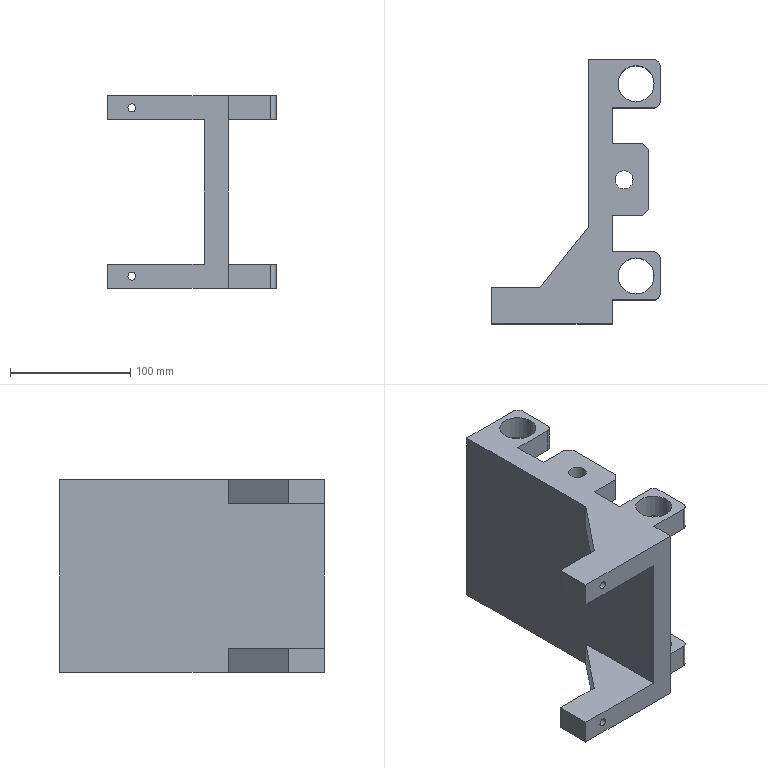Part | STEP file | Mirror 1-1 | 1 solid | 62 faces | box 140 x 220 x 160 mm | volume 939410 mm3 | plane 36 | cylinder 26 | commonest cylinder face diameters 10 x8 30 x8 6.6 x4 14.55 x4 15 x2